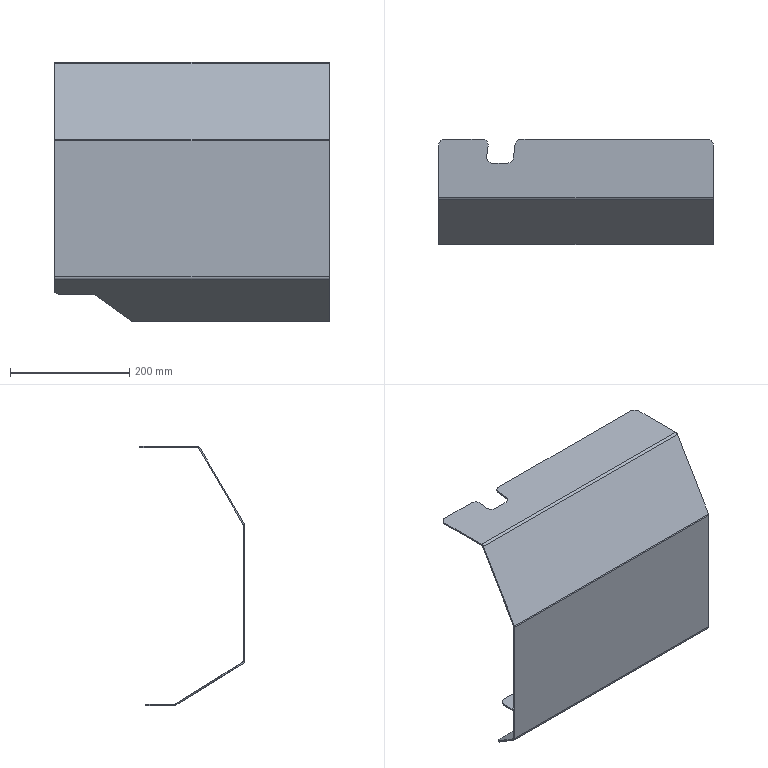Part | SolidWorks | features ICE 3, Fillet 1, FlatPattern 1, SMBaseFlange 1, SheetMetal 1 | 1 solid | 60 faces | box 460 x 176 x 434 mm | volume 663913 mm3 | plane 35 | cylinder 23 | spline 2 | commonest cylinder face diameters 20 x11 5 x4 9.6 x4 12.5 x4